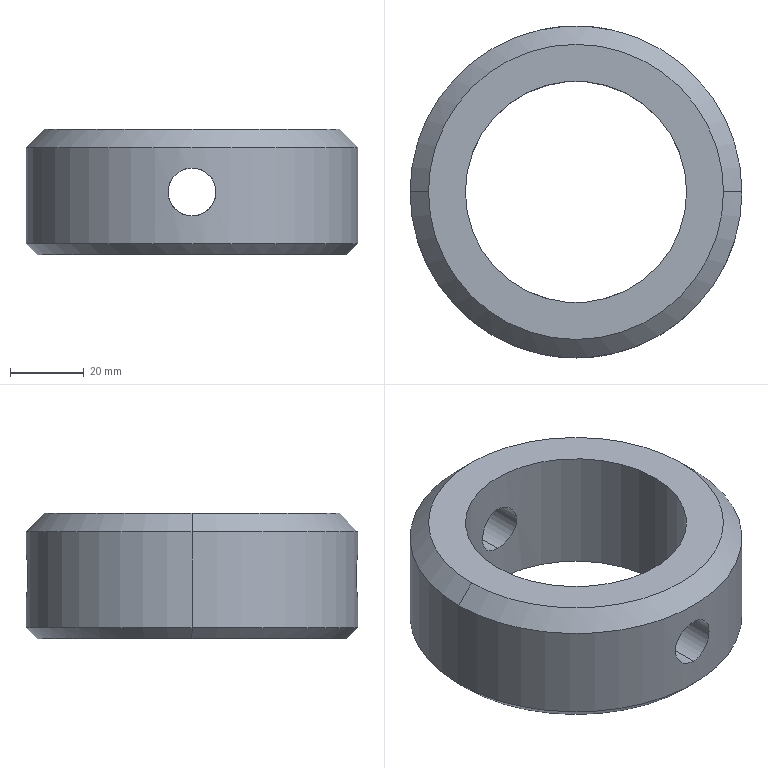Part | SolidWorks | features Chamfer 2, Extrusion 1, ICE 1 | 1 solid | 14 faces | box 90 x 90 x 34 mm | volume 111520 mm3 | cylinder 8 | cone 4 | plane 2 | commonest cylinder face diameters 13 x4 60 x2 90 x2
STEP:
#1=CARTESIAN_POINT('',(-42.,0.,0.));
#2=VERTEX_POINT('',#1);
#3=CARTESIAN_POINT('',(42.,0.,0.));
#4=VERTEX_POINT('',#3);
#5=CARTESIAN_POINT('',(0.,0.,0.));
#6=DIRECTION('',(0.,0.,-1.));
#7=DIRECTION('',(1.,0.,0.));
#8=AXIS2_PLACEMENT_3D('',#5,#6,#7);
#9=CIRCLE('',#8,42.);
#10=EDGE_CURVE('',#2,#4,#9,.T.);
#11=ORIENTED_EDGE('',*,*,#10,.F.);
#12=CARTESIAN_POINT('',(-45.,0.,3.));
#13=VERTEX_POINT('',#12);
#14=CARTESIAN_POINT('',(-45.,0.,3.));
#15=DIRECTION('',(-0.7071,0.,0.7071));
#16=VECTOR('',#15,1000.);
#17=LINE('',#14,#16);
#18=EDGE_CURVE('',#2,#13,#17,.T.);
#19=ORIENTED_EDGE('',*,*,#18,.T.);
#20=CARTESIAN_POINT('',(45.,0.,3.));
#21=VERTEX_POINT('',#20);
#22=CARTESIAN_POINT('',(0.,0.,3.));
#23=DIRECTION('',(0.,0.,1.));
#24=DIRECTION('',(1.,0.,0.));
#25=AXIS2_PLACEMENT_3D('',#22,#23,#24);
#26=CIRCLE('',#25,45.);
#27=EDGE_CURVE('',#21,#13,#26,.T.);
#28=ORIENTED_EDGE('',*,*,#27,.F.);
#29=CARTESIAN_POINT('',(45.,0.,3.));
#30=DIRECTION('',(0.7071,0.,0.7071));
#31=VECTOR('',#30,1000.);
#32=LINE('',#29,#31);
#33=EDGE_CURVE('',#4,#21,#32,.T.);
#34=ORIENTED_EDGE('',*,*,#33,.F.);
#35=EDGE_LOOP('',(#11,#19,#28,#34));
#36=FACE_OUTER_BOUND('',#35,.T.);
#37=CARTESIAN_POINT('',(0.,0.,3.));
#38=DIRECTION('',(0.,0.,1.));
#39=DIRECTION('',(1.,0.,0.));
#40=AXIS2_PLACEMENT_3D('',#37,#38,#39);
#41=CONICAL_SURFACE('',#40,45.,0.7854);
#42=ADVANCED_FACE('',(#36),#41,.T.);
#43=CARTESIAN_POINT('',(40.,0.,34.));
#44=VERTEX_POINT('',#43);
#45=CARTESIAN_POINT('',(-40.,0.,34.));
#46=VERTEX_POINT('',#45);
#47=CARTESIAN_POINT('',(0.,0.,34.));
#48=DIRECTION('',(0.,0.,1.));
#49=DIRECTION('',(1.,0.,0.));
#50=AXIS2_PLACEMENT_3D('',#47,#48,#49);
#51=CIRCLE('',#50,40.);
#52=EDGE_CURVE('',#44,#46,#51,.T.);
#53=ORIENTED_EDGE('',*,*,#52,.F.);
#54=CARTESIAN_POINT('',(45.,0.,29.));
#55=VERTEX_POINT('',#54);
#56=CARTESIAN_POINT('',(40.,0.,34.));
#57=DIRECTION('',(0.7071,0.,-0.7071));
#58=VECTOR('',#57,1000.);
#59=LINE('',#56,#58);
#60=EDGE_CURVE('',#44,#55,#59,.T.);
#61=ORIENTED_EDGE('',*,*,#60,.T.);
#62=CARTESIAN_POINT('',(-45.,0.,29.));
#63=VERTEX_POINT('',#62);
#64=CARTESIAN_POINT('',(0.,0.,29.));
#65=DIRECTION('',(0.,0.,-1.));
#66=DIRECTION('',(1.,0.,0.));
#67=AXIS2_PLACEMENT_3D('',#64,#65,#66);
#68=CIRCLE('',#67,45.);
#69=EDGE_CURVE('',#63,#55,#68,.T.);
#70=ORIENTED_EDGE('',*,*,#69,.F.);
#71=CARTESIAN_POINT('',(-40.,0.,34.));
#72=DIRECTION('',(-0.7071,0.,-0.7071));
#73=VECTOR('',#72,1000.);
#74=LINE('',#71,#73);
#75=EDGE_CURVE('',#46,#63,#74,.T.);
#76=ORIENTED_EDGE('',*,*,#75,.F.);
#77=EDGE_LOOP('',(#53,#61,#70,#76));
#78=FACE_OUTER_BOUND('',#77,.T.);
#79=CARTESIAN_POINT('',(0.,0.,34.));
#80=DIRECTION('',(0.,0.,-1.));
#81=DIRECTION('',(-1.,0.,0.));
#82=AXIS2_PLACEMENT_3D('',#79,#80,#81);
#83=CONICAL_SURFACE('',#82,40.,0.7854);
#84=ADVANCED_FACE('',(#78),#83,.T.);
#85=CARTESIAN_POINT('',(0.,-45.,10.5));
#86=VERTEX_POINT('',#85);
#87=CARTESIAN_POINT('',(0.,-45.,23.5));
#88=VERTEX_POINT('',#87);
#89=CARTESIAN_POINT('',(0.,-45.,10.5));
#90=CARTESIAN_POINT('',(-0.4244,-45.,10.5));
#91=CARTESIAN_POINT('',(-0.8466,-44.994,10.541));
#92=CARTESIAN_POINT('',(-1.477,-44.976,10.666));
#93=CARTESIAN_POINT('',(-1.685,-44.969,10.719));
#94=CARTESIAN_POINT('',(-2.092,-44.952,10.842));
#95=CARTESIAN_POINT('',(-2.491,-44.932,10.985));
#96=CARTESIAN_POINT('',(-2.875,-44.908,11.166));
#97=CARTESIAN_POINT('',(-3.25,-44.883,11.367));
#98=CARTESIAN_POINT('',(-3.434,-44.869,11.477));
#99=CARTESIAN_POINT('',(-3.967,-44.826,11.833));
#100=CARTESIAN_POINT('',(-4.293,-44.796,12.101));
#101=CARTESIAN_POINT('',(-4.893,-44.734,12.7));
#102=CARTESIAN_POINT('',(-5.167,-44.703,13.034));
#103=CARTESIAN_POINT('',(-5.639,-44.646,13.739));
#104=CARTESIAN_POINT('',(-5.839,-44.62,14.112));
#105=CARTESIAN_POINT('',(-6.084,-44.587,14.702));
#106=CARTESIAN_POINT('',(-6.157,-44.577,14.905));
#107=CARTESIAN_POINT('',(-6.281,-44.56,15.313));
#108=CARTESIAN_POINT('',(-6.333,-44.552,15.519));
#109=CARTESIAN_POINT('',(-6.457,-44.534,16.143));
#110=CARTESIAN_POINT('',(-6.5,-44.528,16.566));
#111=CARTESIAN_POINT('',(-6.5,-44.528,17.425));
#112=CARTESIAN_POINT('',(-6.458,-44.534,17.848));
#113=CARTESIAN_POINT('',(-6.335,-44.552,18.472));
#114=CARTESIAN_POINT('',(-6.283,-44.559,18.678));
#115=CARTESIAN_POINT('',(-6.16,-44.576,19.087));
#116=CARTESIAN_POINT('',(-6.087,-44.586,19.29));
#117=CARTESIAN_POINT('',(-5.843,-44.619,19.88));
#118=CARTESIAN_POINT('',(-5.643,-44.645,20.253));
#119=CARTESIAN_POINT('',(-5.172,-44.702,20.96));
#120=CARTESIAN_POINT('',(-4.898,-44.734,21.294));
#121=CARTESIAN_POINT('',(-4.3,-44.795,21.893));
#122=CARTESIAN_POINT('',(-3.974,-44.826,22.162));
#123=CARTESIAN_POINT('',(-3.263,-44.883,22.638));
#124=CARTESIAN_POINT('',(-2.887,-44.909,22.839));
#125=CARTESIAN_POINT('',(-2.3,-44.942,23.083));
#126=CARTESIAN_POINT('',(-2.101,-44.951,23.155));
#127=CARTESIAN_POINT('',(-1.694,-44.969,23.279));
#128=CARTESIAN_POINT('',(-1.485,-44.976,23.332));
#129=CARTESIAN_POINT('',(-0.8549,-44.994,23.458));
#130=CARTESIAN_POINT('',(-0.43,-45.,23.5));
#131=CARTESIAN_POINT('',(0.,-45.,23.5));
#132=B_SPLINE_CURVE_WITH_KNOTS('',3,(#89,#90,#91,#92,#93,#94,#95,#96,#97,#98,#99,#100,#101,#102,#103,#104,#105,#106,#107,#108,#109,#110,#111,#112,#113,#114,#115,#116,#117,#118,#119,#120,#121,#122,#123,#124,#125,#126,#127,#128,#129,#130,#131),.UNSPECIFIED.,.F.,.F.,(4,2,2,1,2,2,2,2,2,2,2,2,2,2,2,2,2,2,2,2,2,4),(0.02035,0.02162,0.02226,0.02289,0.02353,0.02416,0.02543,0.02671,0.02798,0.02861,0.02925,0.03052,0.03179,0.03243,0.03306,0.03433,0.03561,0.03688,0.03815,0.03878,0.03942,0.04069),.UNSPECIFIED.);
#133=EDGE_CURVE('',#86,#88,#132,.T.);
#134=ORIENTED_EDGE('',*,*,#133,.F.);
#135=CARTESIAN_POINT('',(0.,-30.,10.5));
#136=VERTEX_POINT('',#135);
#137=CARTESIAN_POINT('',(0.,-45.,10.5));
#138=DIRECTION('',(0.,1.,0.));
#139=VECTOR('',#138,1000.);
#140=LINE('',#137,#139);
#141=EDGE_CURVE('',#86,#136,#140,.T.);
#142=ORIENTED_EDGE('',*,*,#141,.T.);
#143=CARTESIAN_POINT('',(0.,-30.,23.5));
#144=VERTEX_POINT('',#143);
#145=CARTESIAN_POINT('',(0.,-30.,10.5));
#146=CARTESIAN_POINT('',(-0.4248,-30.,10.5));
#147=CARTESIAN_POINT('',(-0.848,-29.991,10.541));
#148=CARTESIAN_POINT('',(-1.691,-29.955,10.709));
#149=CARTESIAN_POINT('',(-2.099,-29.929,10.834));
#150=CARTESIAN_POINT('',(-2.686,-29.88,11.077));
#151=CARTESIAN_POINT('',(-2.877,-29.862,11.168));
#152=CARTESIAN_POINT('',(-3.253,-29.824,11.369));
#153=CARTESIAN_POINT('',(-3.438,-29.803,11.479));
#154=CARTESIAN_POINT('',(-3.968,-29.739,11.834));
#155=CARTESIAN_POINT('',(-4.294,-29.693,12.102));
#156=CARTESIAN_POINT('',(-4.894,-29.6,12.701));
#157=CARTESIAN_POINT('',(-5.167,-29.553,13.034));
#158=CARTESIAN_POINT('',(-5.638,-29.466,13.737));
#159=CARTESIAN_POINT('',(-5.838,-29.427,14.11));
#160=CARTESIAN_POINT('',(-6.084,-29.377,14.702));
#161=CARTESIAN_POINT('',(-6.157,-29.362,14.904));
#162=CARTESIAN_POINT('',(-6.281,-29.335,15.312));
#163=CARTESIAN_POINT('',(-6.384,-29.313,15.723));
#164=CARTESIAN_POINT('',(-6.447,-29.299,16.143));
#165=CARTESIAN_POINT('',(-6.489,-29.29,16.567));
#166=CARTESIAN_POINT('',(-6.5,-29.287,16.783));
#167=CARTESIAN_POINT('',(-6.5,-29.287,17.426));
#168=CARTESIAN_POINT('',(-6.458,-29.297,17.849));
#169=CARTESIAN_POINT('',(-6.293,-29.333,18.682));
#170=CARTESIAN_POINT('',(-6.167,-29.36,19.097));
#171=CARTESIAN_POINT('',(-5.842,-29.426,19.882));
#172=CARTESIAN_POINT('',(-5.642,-29.466,20.255));
#173=CARTESIAN_POINT('',(-5.288,-29.531,20.786));
#174=CARTESIAN_POINT('',(-5.16,-29.553,20.959));
#175=CARTESIAN_POINT('',(-4.89,-29.599,21.287));
#176=CARTESIAN_POINT('',(-4.748,-29.622,21.444));
#177=CARTESIAN_POINT('',(-4.301,-29.692,21.892));
#178=CARTESIAN_POINT('',(-3.973,-29.738,22.162));
#179=CARTESIAN_POINT('',(-3.262,-29.824,22.638));
#180=CARTESIAN_POINT('',(-2.889,-29.863,22.838));
#181=CARTESIAN_POINT('',(-2.303,-29.912,23.082));
#182=CARTESIAN_POINT('',(-2.103,-29.927,23.154));
#183=CARTESIAN_POINT('',(-1.694,-29.953,23.279));
#184=CARTESIAN_POINT('',(-1.485,-29.964,23.332));
#185=CARTESIAN_POINT('',(-0.8557,-29.991,23.458));
#186=CARTESIAN_POINT('',(-0.4307,-30.,23.5));
#187=CARTESIAN_POINT('',(0.,-30.,23.5));
#188=B_SPLINE_CURVE_WITH_KNOTS('',3,(#145,#146,#147,#148,#149,#150,#151,#152,#153,#154,#155,#156,#157,#158,#159,#160,#161,#162,#163,#164,#165,#166,#167,#168,#169,#170,#171,#172,#173,#174,#175,#176,#177,#178,#179,#180,#181,#182,#183,#184,#185,#186,#187),.UNSPECIFIED.,.F.,.F.,(4,2,2,2,2,2,2,2,2,1,2,2,2,2,2,2,2,2,2,2,2,4),(0.02038,0.02166,0.02293,0.02357,0.0242,0.02548,0.02675,0.02802,0.02866,0.0293,0.02993,0.03057,0.03184,0.03312,0.03439,0.03503,0.03567,0.03694,0.03821,0.03885,0.03949,0.04076),.UNSPECIFIED.);
#189=EDGE_CURVE('',#136,#144,#188,.T.);
#190=ORIENTED_EDGE('',*,*,#189,.T.);
#191=CARTESIAN_POINT('',(0.,-45.,23.5));
#192=DIRECTION('',(0.,1.,0.));
#193=VECTOR('',#192,1000.);
#194=LINE('',#191,#193);
#195=EDGE_CURVE('',#88,#144,#194,.T.);
#196=ORIENTED_EDGE('',*,*,#195,.F.);
#197=EDGE_LOOP('',(#134,#142,#190,#196));
#198=FACE_OUTER_BOUND('',#197,.T.);
#199=CARTESIAN_POINT('',(0.,-45.,17.));
#200=DIRECTION('',(0.,1.,0.));
#201=DIRECTION('',(0.,0.,1.));
#202=AXIS2_PLACEMENT_3D('',#199,#200,#201);
#203=CYLINDRICAL_SURFACE('',#202,6.5);
#204=ADVANCED_FACE('',(#198),#203,.F.);
#205=CARTESIAN_POINT('',(0.,30.,23.5));
#206=VERTEX_POINT('',#205);
#207=CARTESIAN_POINT('',(0.,30.,10.5));
#208=VERTEX_POINT('',#207);
#209=CARTESIAN_POINT('',(0.,30.,23.5));
#210=CARTESIAN_POINT('',(-0.4308,30.,23.5));
#211=CARTESIAN_POINT('',(-0.8542,29.991,23.458));
#212=CARTESIAN_POINT('',(-1.479,29.964,23.333));
#213=CARTESIAN_POINT('',(-1.685,29.953,23.281));
#214=CARTESIAN_POINT('',(-2.094,29.928,23.157));
#215=CARTESIAN_POINT('',(-2.297,29.913,23.084));
#216=CARTESIAN_POINT('',(-2.887,29.863,22.839));
#217=CARTESIAN_POINT('',(-3.26,29.824,22.639));
#218=CARTESIAN_POINT('',(-3.966,29.739,22.168));
#219=CARTESIAN_POINT('',(-4.299,29.692,21.894));
#220=CARTESIAN_POINT('',(-4.896,29.599,21.296));
#221=CARTESIAN_POINT('',(-5.165,29.553,20.97));
#222=CARTESIAN_POINT('',(-5.64,29.466,20.259));
#223=CARTESIAN_POINT('',(-5.841,29.426,19.883));
#224=CARTESIAN_POINT('',(-6.084,29.377,19.297));
#225=CARTESIAN_POINT('',(-6.156,29.362,19.097));
#226=CARTESIAN_POINT('',(-6.28,29.335,18.69));
#227=CARTESIAN_POINT('',(-6.333,29.324,18.48));
#228=CARTESIAN_POINT('',(-6.458,29.297,17.851));
#229=CARTESIAN_POINT('',(-6.5,29.287,17.428));
#230=CARTESIAN_POINT('',(-6.5,29.287,16.577));
#231=CARTESIAN_POINT('',(-6.458,29.297,16.145));
#232=CARTESIAN_POINT('',(-6.291,29.333,15.31));
#233=CARTESIAN_POINT('',(-6.168,29.36,14.905));
#234=CARTESIAN_POINT('',(-5.923,29.41,14.313));
#235=CARTESIAN_POINT('',(-5.83,29.428,14.118));
#236=CARTESIAN_POINT('',(-5.629,29.467,13.743));
#237=CARTESIAN_POINT('',(-5.52,29.488,13.562));
#238=CARTESIAN_POINT('',(-5.168,29.553,13.035));
#239=CARTESIAN_POINT('',(-4.897,29.599,12.705));
#240=CARTESIAN_POINT('',(-4.294,29.693,12.101));
#241=CARTESIAN_POINT('',(-3.967,29.739,11.834));
#242=CARTESIAN_POINT('',(-3.44,29.803,11.481));
#243=CARTESIAN_POINT('',(-3.258,29.823,11.371));
#244=CARTESIAN_POINT('',(-2.881,29.862,11.169));
#245=CARTESIAN_POINT('',(-2.687,29.88,11.077));
#246=CARTESIAN_POINT('',(-2.098,29.929,10.833));
#247=CARTESIAN_POINT('',(-1.692,29.955,10.71));
#248=CARTESIAN_POINT('',(-1.065,29.982,10.584));
#249=CARTESIAN_POINT('',(-0.852,29.989,10.553));
#250=CARTESIAN_POINT('',(-0.4254,29.998,10.51));
#251=CARTESIAN_POINT('',(-0.2125,30.,10.5));
#252=CARTESIAN_POINT('',(0.,30.,10.5));
#253=B_SPLINE_CURVE_WITH_KNOTS('',3,(#209,#210,#211,#212,#213,#214,#215,#216,#217,#218,#219,#220,#221,#222,#223,#224,#225,#226,#227,#228,#229,#230,#231,#232,#233,#234,#235,#236,#237,#238,#239,#240,#241,#242,#243,#244,#245,#246,#247,#248,#249,#250,#251,#252),.UNSPECIFIED.,.F.,.F.,(4,2,2,2,2,2,2,2,2,2,2,2,2,2,2,2,2,2,2,2,2,4),(0.,0.001274,0.001911,0.002548,0.003822,0.005096,0.00637,0.007643,0.00828,0.008917,0.01019,0.01147,0.01274,0.01338,0.01401,0.01529,0.01656,0.0172,0.01783,0.01911,0.01975,0.02038),.UNSPECIFIED.);
#254=EDGE_CURVE('',#206,#208,#253,.T.);
#255=ORIENTED_EDGE('',*,*,#254,.T.);
#256=CARTESIAN_POINT('',(0.,45.,10.5));
#257=VERTEX_POINT('',#256);
#258=CARTESIAN_POINT('',(0.,-45.,10.5));
#259=DIRECTION('',(0.,1.,0.));
#260=VECTOR('',#259,1000.);
#261=LINE('',#258,#260);
#262=EDGE_CURVE('',#208,#257,#261,.T.);
#263=ORIENTED_EDGE('',*,*,#262,.T.);
#264=CARTESIAN_POINT('',(0.,45.,23.5));
#265=VERTEX_POINT('',#264);
#266=CARTESIAN_POINT('',(0.,45.,23.5));
#267=CARTESIAN_POINT('',(-0.4301,45.,23.5));
#268=CARTESIAN_POINT('',(-0.8529,44.994,23.458));
#269=CARTESIAN_POINT('',(-1.477,44.976,23.334));
#270=CARTESIAN_POINT('',(-1.683,44.969,23.282));
#271=CARTESIAN_POINT('',(-2.091,44.952,23.158));
#272=CARTESIAN_POINT('',(-2.294,44.942,23.085));
#273=CARTESIAN_POINT('',(-2.885,44.909,22.84));
#274=CARTESIAN_POINT('',(-3.258,44.883,22.641));
#275=CARTESIAN_POINT('',(-3.964,44.826,22.169));
#276=CARTESIAN_POINT('',(-4.298,44.795,21.895));
#277=CARTESIAN_POINT('',(-4.897,44.734,21.296));
#278=CARTESIAN_POINT('',(-5.165,44.703,20.969));
#279=CARTESIAN_POINT('',(-5.522,44.66,20.436));
#280=CARTESIAN_POINT('',(-5.632,44.646,20.252));
#281=CARTESIAN_POINT('',(-5.833,44.621,19.877));
#282=CARTESIAN_POINT('',(-6.014,44.597,19.494));
#283=CARTESIAN_POINT('',(-6.157,44.577,19.095));
#284=CARTESIAN_POINT('',(-6.281,44.56,18.688));
#285=CARTESIAN_POINT('',(-6.333,44.552,18.479));
#286=CARTESIAN_POINT('',(-6.458,44.534,17.849));
#287=CARTESIAN_POINT('',(-6.5,44.528,17.427));
#288=CARTESIAN_POINT('',(-6.5,44.528,16.578));
#289=CARTESIAN_POINT('',(-6.458,44.534,16.147));
#290=CARTESIAN_POINT('',(-6.291,44.558,15.312));
#291=CARTESIAN_POINT('',(-6.169,44.576,14.907));
#292=CARTESIAN_POINT('',(-5.924,44.608,14.316));
#293=CARTESIAN_POINT('',(-5.832,44.621,14.121));
#294=CARTESIAN_POINT('',(-5.631,44.646,13.745));
#295=CARTESIAN_POINT('',(-5.521,44.66,13.564));
#296=CARTESIAN_POINT('',(-5.169,44.703,13.036));
#297=CARTESIAN_POINT('',(-4.899,44.734,12.707));
#298=CARTESIAN_POINT('',(-4.294,44.796,12.101));
#299=CARTESIAN_POINT('',(-3.966,44.826,11.833));
#300=CARTESIAN_POINT('',(-3.438,44.869,11.48));
#301=CARTESIAN_POINT('',(-3.256,44.882,11.37));
#302=CARTESIAN_POINT('',(-2.88,44.908,11.169));
#303=CARTESIAN_POINT('',(-2.685,44.92,11.077));
#304=CARTESIAN_POINT('',(-2.095,44.953,10.832));
#305=CARTESIAN_POINT('',(-1.69,44.97,10.709));
#306=CARTESIAN_POINT('',(-0.8557,44.994,10.543));
#307=CARTESIAN_POINT('',(-0.4245,45.,10.5));
#308=CARTESIAN_POINT('',(0.,45.,10.5));
#309=B_SPLINE_CURVE_WITH_KNOTS('',3,(#266,#267,#268,#269,#270,#271,#272,#273,#274,#275,#276,#277,#278,#279,#280,#281,#282,#283,#284,#285,#286,#287,#288,#289,#290,#291,#292,#293,#294,#295,#296,#297,#298,#299,#300,#301,#302,#303,#304,#305,#306,#307,#308),.UNSPECIFIED.,.F.,.F.,(4,2,2,2,2,2,2,2,1,2,2,2,2,2,2,2,2,2,2,2,2,4),(0.,0.001272,0.001908,0.002544,0.003815,0.005087,0.006359,0.006995,0.007631,0.008267,0.008903,0.01017,0.01145,0.01272,0.01335,0.01399,0.01526,0.01653,0.01717,0.01781,0.01908,0.02035),.UNSPECIFIED.);
#310=EDGE_CURVE('',#265,#257,#309,.T.);
#311=ORIENTED_EDGE('',*,*,#310,.F.);
#312=CARTESIAN_POINT('',(0.,-45.,23.5));
#313=DIRECTION('',(0.,1.,0.));
#314=VECTOR('',#313,1000.);
#315=LINE('',#312,#314);
#316=EDGE_CURVE('',#206,#265,#315,.T.);
#317=ORIENTED_EDGE('',*,*,#316,.F.);
#318=EDGE_LOOP('',(#255,#263,#311,#317));
#319=FACE_OUTER_BOUND('',#318,.T.);
#320=CARTESIAN_POINT('',(0.,-45.,17.));
#321=DIRECTION('',(0.,1.,0.));
#322=DIRECTION('',(0.,0.,1.));
#323=AXIS2_PLACEMENT_3D('',#320,#321,#322);
#324=CYLINDRICAL_SURFACE('',#323,6.5);
#325=ADVANCED_FACE('',(#319),#324,.F.);
#326=CARTESIAN_POINT('',(0.,-30.,23.5));
#327=CARTESIAN_POINT('',(0.4308,-30.,23.5));
#328=CARTESIAN_POINT('',(0.8542,-29.991,23.458));
#329=CARTESIAN_POINT('',(1.479,-29.964,23.333));
#330=CARTESIAN_POINT('',(1.685,-29.953,23.281));
#331=CARTESIAN_POINT('',(2.094,-29.928,23.157));
#332=CARTESIAN_POINT('',(2.297,-29.913,23.084));
#333=CARTESIAN_POINT('',(2.887,-29.863,22.839));
#334=CARTESIAN_POINT('',(3.26,-29.824,22.639));
#335=CARTESIAN_POINT('',(3.966,-29.739,22.168));
#336=CARTESIAN_POINT('',(4.299,-29.692,21.894));
#337=CARTESIAN_POINT('',(4.896,-29.599,21.296));
#338=CARTESIAN_POINT('',(5.165,-29.553,20.97));
#339=CARTESIAN_POINT('',(5.64,-29.466,20.259));
#340=CARTESIAN_POINT('',(5.841,-29.426,19.883));
#341=CARTESIAN_POINT('',(6.084,-29.377,19.297));
#342=CARTESIAN_POINT('',(6.156,-29.362,19.097));
#343=CARTESIAN_POINT('',(6.28,-29.335,18.69));
#344=CARTESIAN_POINT('',(6.333,-29.324,18.48));
#345=CARTESIAN_POINT('',(6.458,-29.297,17.851));
#346=CARTESIAN_POINT('',(6.5,-29.287,17.428));
#347=CARTESIAN_POINT('',(6.5,-29.287,16.577));
#348=CARTESIAN_POINT('',(6.458,-29.297,16.145));
#349=CARTESIAN_POINT('',(6.291,-29.333,15.31));
#350=CARTESIAN_POINT('',(6.168,-29.36,14.905));
#351=CARTESIAN_POINT('',(5.923,-29.41,14.313));
#352=CARTESIAN_POINT('',(5.83,-29.428,14.118));
#353=CARTESIAN_POINT('',(5.629,-29.467,13.743));
#354=CARTESIAN_POINT('',(5.52,-29.488,13.562));
#355=CARTESIAN_POINT('',(5.168,-29.553,13.035));
#356=CARTESIAN_POINT('',(4.897,-29.599,12.705));
#357=CARTESIAN_POINT('',(4.294,-29.693,12.101));
#358=CARTESIAN_POINT('',(3.967,-29.739,11.834));
#359=CARTESIAN_POINT('',(3.44,-29.803,11.481));
#360=CARTESIAN_POINT('',(3.258,-29.823,11.371));
#361=CARTESIAN_POINT('',(2.881,-29.862,11.169));
#362=CARTESIAN_POINT('',(2.687,-29.88,11.077));
#363=CARTESIAN_POINT('',(2.098,-29.929,10.833));
#364=CARTESIAN_POINT('',(1.692,-29.955,10.71));
#365=CARTESIAN_POINT('',(1.065,-29.982,10.584));
#366=CARTESIAN_POINT('',(0.852,-29.989,10.553));
#367=CARTESIAN_POINT('',(0.4254,-29.998,10.51));
#368=CARTESIAN_POINT('',(0.2125,-30.,10.5));
#369=CARTESIAN_POINT('',(0.,-30.,10.5));
#370=B_SPLINE_CURVE_WITH_KNOTS('',3,(#326,#327,#328,#329,#330,#331,#332,#333,#334,#335,#336,#337,#338,#339,#340,#341,#342,#343,#344,#345,#346,#347,#348,#349,#350,#351,#352,#353,#354,#355,#356,#357,#358,#359,#360,#361,#362,#363,#364,#365,#366,#367,#368,#369),.UNSPECIFIED.,.F.,.F.,(4,2,2,2,2,2,2,2,2,2,2,2,2,2,2,2,2,2,2,2,2,4),(0.,0.001274,0.001911,0.002548,0.003822,0.005096,0.00637,0.007643,0.00828,0.008917,0.01019,0.01147,0.01274,0.01338,0.01401,0.01529,0.01656,0.0172,0.01783,0.01911,0.01975,0.02038),.UNSPECIFIED.);
#371=EDGE_CURVE('',#144,#136,#370,.T.);
#372=ORIENTED_EDGE('',*,*,#371,.F.);
#373=ORIENTED_EDGE('',*,*,#189,.F.);
#374=EDGE_LOOP('',(#372,#373));
#375=FACE_BOUND('',#374,.T.);
#376=CARTESIAN_POINT('',(-30.,0.,34.));
#377=VERTEX_POINT('',#376);
#378=CARTESIAN_POINT('',(30.,0.,34.));
#379=VERTEX_POINT('',#378);
#380=CARTESIAN_POINT('',(0.,0.,34.));
#381=DIRECTION('',(0.,0.,1.));
#382=DIRECTION('',(1.,0.,0.));
#383=AXIS2_PLACEMENT_3D('',#380,#381,#382);
#384=CIRCLE('',#383,30.);
#385=EDGE_CURVE('',#377,#379,#384,.T.);
#386=ORIENTED_EDGE('',*,*,#385,.T.);
#387=CARTESIAN_POINT('',(30.,0.,0.));
#388=VERTEX_POINT('',#387);
#389=CARTESIAN_POINT('',(30.,0.,34.));
#390=DIRECTION('',(0.,0.,-1.));
#391=VECTOR('',#390,1000.);
#392=LINE('',#389,#391);
#393=EDGE_CURVE('',#379,#388,#392,.T.);
#394=ORIENTED_EDGE('',*,*,#393,.T.);
#395=CARTESIAN_POINT('',(-30.,0.,0.));
#396=VERTEX_POINT('',#395);
#397=CARTESIAN_POINT('',(0.,0.,0.));
#398=DIRECTION('',(0.,0.,1.));
#399=DIRECTION('',(1.,0.,0.));
#400=AXIS2_PLACEMENT_3D('',#397,#398,#399);
#401=CIRCLE('',#400,30.);
#402=EDGE_CURVE('',#396,#388,#401,.T.);
#403=ORIENTED_EDGE('',*,*,#402,.F.);
#404=CARTESIAN_POINT('',(-30.,0.,34.));
#405=DIRECTION('',(0.,0.,-1.));
#406=VECTOR('',#405,1000.);
#407=LINE('',#404,#406);
#408=EDGE_CURVE('',#377,#396,#407,.T.);
#409=ORIENTED_EDGE('',*,*,#408,.F.);
#410=EDGE_LOOP('',(#386,#394,#403,#409));
#411=FACE_OUTER_BOUND('',#410,.T.);
#412=CARTESIAN_POINT('',(0.,0.,34.));
#413=DIRECTION('',(0.,0.,-1.));
#414=DIRECTION('',(-1.,0.,0.));
#415=AXIS2_PLACEMENT_3D('',#412,#413,#414);
#416=CYLINDRICAL_SURFACE('',#415,30.);
#417=ADVANCED_FACE('',(#375,#411),#416,.F.);
#418=ORIENTED_EDGE('',*,*,#310,.T.);
#419=CARTESIAN_POINT('',(0.,45.,10.5));
#420=CARTESIAN_POINT('',(0.4244,45.,10.5));
#421=CARTESIAN_POINT('',(0.8466,44.994,10.541));
#422=CARTESIAN_POINT('',(1.477,44.976,10.666));
#423=CARTESIAN_POINT('',(1.685,44.969,10.719));
#424=CARTESIAN_POINT('',(2.092,44.952,10.842));
#425=CARTESIAN_POINT('',(2.491,44.932,10.985));
#426=CARTESIAN_POINT('',(2.875,44.908,11.166));
#427=CARTESIAN_POINT('',(3.25,44.883,11.367));
#428=CARTESIAN_POINT('',(3.434,44.869,11.477));
#429=CARTESIAN_POINT('',(3.967,44.826,11.833));
#430=CARTESIAN_POINT('',(4.293,44.796,12.101));
#431=CARTESIAN_POINT('',(4.893,44.734,12.7));
#432=CARTESIAN_POINT('',(5.167,44.703,13.034));
#433=CARTESIAN_POINT('',(5.639,44.646,13.739));
#434=CARTESIAN_POINT('',(5.839,44.62,14.112));
#435=CARTESIAN_POINT('',(6.084,44.587,14.702));
#436=CARTESIAN_POINT('',(6.157,44.577,14.905));
#437=CARTESIAN_POINT('',(6.281,44.56,15.313));
#438=CARTESIAN_POINT('',(6.333,44.552,15.519));
#439=CARTESIAN_POINT('',(6.457,44.534,16.143));
#440=CARTESIAN_POINT('',(6.5,44.528,16.566));
#441=CARTESIAN_POINT('',(6.5,44.528,17.425));
#442=CARTESIAN_POINT('',(6.458,44.534,17.848));
#443=CARTESIAN_POINT('',(6.335,44.552,18.472));
#444=CARTESIAN_POINT('',(6.283,44.559,18.678));
#445=CARTESIAN_POINT('',(6.16,44.576,19.087));
#446=CARTESIAN_POINT('',(6.087,44.586,19.29));
#447=CARTESIAN_POINT('',(5.843,44.619,19.88));
#448=CARTESIAN_POINT('',(5.643,44.645,20.253));
#449=CARTESIAN_POINT('',(5.172,44.702,20.96));
#450=CARTESIAN_POINT('',(4.898,44.734,21.294));
#451=CARTESIAN_POINT('',(4.3,44.795,21.893));
#452=CARTESIAN_POINT('',(3.974,44.826,22.162));
#453=CARTESIAN_POINT('',(3.263,44.883,22.638));
#454=CARTESIAN_POINT('',(2.887,44.909,22.839));
#455=CARTESIAN_POINT('',(2.3,44.942,23.083));
#456=CARTESIAN_POINT('',(2.101,44.951,23.155));
#457=CARTESIAN_POINT('',(1.694,44.969,23.279));
#458=CARTESIAN_POINT('',(1.485,44.976,23.332));
#459=CARTESIAN_POINT('',(0.8549,44.994,23.458));
#460=CARTESIAN_POINT('',(0.43,45.,23.5));
#461=CARTESIAN_POINT('',(0.,45.,23.5));
#462=B_SPLINE_CURVE_WITH_KNOTS('',3,(#419,#420,#421,#422,#423,#424,#425,#426,#427,#428,#429,#430,#431,#432,#433,#434,#435,#436,#437,#438,#439,#440,#441,#442,#443,#444,#445,#446,#447,#448,#449,#450,#451,#452,#453,#454,#455,#456,#457,#458,#459,#460,#461),.UNSPECIFIED.,.F.,.F.,(4,2,2,1,2,2,2,2,2,2,2,2,2,2,2,2,2,2,2,2,2,4),(0.02035,0.02162,0.02226,0.02289,0.02353,0.02416,0.02543,0.02671,0.02798,0.02861,0.02925,0.03052,0.03179,0.03243,0.03306,0.03433,0.03561,0.03688,0.03815,0.03878,0.03942,0.04069),.UNSPECIFIED.);
#463=EDGE_CURVE('',#257,#265,#462,.T.);
#464=ORIENTED_EDGE('',*,*,#463,.T.);
#465=EDGE_LOOP('',(#418,#464));
#466=FACE_BOUND('',#465,.T.);
#467=ORIENTED_EDGE('',*,*,#69,.T.);
#468=CARTESIAN_POINT('',(45.,0.,34.));
#469=DIRECTION('',(0.,0.,-1.));
#470=VECTOR('',#469,1000.);
#471=LINE('',#468,#470);
#472=EDGE_CURVE('',#55,#21,#471,.T.);
#473=ORIENTED_EDGE('',*,*,#472,.T.);
#474=ORIENTED_EDGE('',*,*,#27,.T.);
#475=CARTESIAN_POINT('',(-45.,0.,34.));
#476=DIRECTION('',(0.,0.,-1.));
#477=VECTOR('',#476,1000.);
#478=LINE('',#475,#477);
#479=EDGE_CURVE('',#63,#13,#478,.T.);
#480=ORIENTED_EDGE('',*,*,#479,.F.);
#481=EDGE_LOOP('',(#467,#473,#474,#480));
#482=FACE_OUTER_BOUND('',#481,.T.);
#483=CARTESIAN_POINT('',(0.,0.,34.));
#484=DIRECTION('',(0.,0.,-1.));
#485=DIRECTION('',(-1.,0.,0.));
#486=AXIS2_PLACEMENT_3D('',#483,#484,#485);
#487=CYLINDRICAL_SURFACE('',#486,45.);
#488=ADVANCED_FACE('',(#466,#482),#487,.T.);
#489=CARTESIAN_POINT('',(0.,0.,34.));
#490=DIRECTION('',(0.,0.,1.));
#491=DIRECTION('',(1.,0.,0.));
#492=AXIS2_PLACEMENT_3D('',#489,#490,#491);
#493=CIRCLE('',#492,40.);
#494=EDGE_CURVE('',#46,#44,#493,.T.);
#495=ORIENTED_EDGE('',*,*,#494,.T.);
#496=ORIENTED_EDGE('',*,*,#52,.T.);
#497=EDGE_LOOP('',(#495,#496));
#498=FACE_OUTER_BOUND('',#497,.T.);
#499=ORIENTED_EDGE('',*,*,#385,.F.);
#500=CARTESIAN_POINT('',(0.,0.,34.));
#501=DIRECTION('',(0.,0.,1.));
#502=DIRECTION('',(1.,0.,0.));
#503=AXIS2_PLACEMENT_3D('',#500,#501,#502);
#504=CIRCLE('',#503,30.);
#505=EDGE_CURVE('',#379,#377,#504,.T.);
#506=ORIENTED_EDGE('',*,*,#505,.F.);
#507=EDGE_LOOP('',(#499,#506));
#508=FACE_BOUND('',#507,.T.);
#509=CARTESIAN_POINT('',(0.,0.,34.));
#510=DIRECTION('',(0.,0.,1.));
#511=DIRECTION('',(1.,0.,0.));
#512=AXIS2_PLACEMENT_3D('',#509,#510,#511);
#513=PLANE('',#512);
#514=ADVANCED_FACE('',(#498,#508),#513,.T.);
#515=CARTESIAN_POINT('',(0.,0.,0.));
#516=DIRECTION('',(0.,0.,-1.));
#517=DIRECTION('',(1.,0.,0.));
#518=AXIS2_PLACEMENT_3D('',#515,#516,#517);
#519=CIRCLE('',#518,42.);
#520=EDGE_CURVE('',#4,#2,#519,.T.);
#521=ORIENTED_EDGE('',*,*,#520,.T.);
#522=ORIENTED_EDGE('',*,*,#10,.T.);
#523=EDGE_LOOP('',(#521,#522));
#524=FACE_OUTER_BOUND('',#523,.T.);
#525=ORIENTED_EDGE('',*,*,#402,.T.);
#526=CARTESIAN_POINT('',(0.,0.,0.));
#527=DIRECTION('',(0.,0.,1.));
#528=DIRECTION('',(1.,0.,0.));
#529=AXIS2_PLACEMENT_3D('',#526,#527,#528);
#530=CIRCLE('',#529,30.);
#531=EDGE_CURVE('',#388,#396,#530,.T.);
#532=ORIENTED_EDGE('',*,*,#531,.T.);
#533=EDGE_LOOP('',(#525,#532));
#534=FACE_BOUND('',#533,.T.);
#535=CARTESIAN_POINT('',(0.,0.,0.));
#536=DIRECTION('',(0.,0.,1.));
#537=DIRECTION('',(1.,0.,0.));
#538=AXIS2_PLACEMENT_3D('',#535,#536,#537);
#539=PLANE('',#538);
#540=ADVANCED_FACE('',(#524,#534),#539,.F.);
#541=ORIENTED_EDGE('',*,*,#472,.F.);
#542=CARTESIAN_POINT('',(0.,0.,29.));
#543=DIRECTION('',(0.,0.,-1.));
#544=DIRECTION('',(1.,0.,0.));
#545=AXIS2_PLACEMENT_3D('',#542,#543,#544);
#546=CIRCLE('',#545,45.);
#547=EDGE_CURVE('',#55,#63,#546,.T.);
#548=ORIENTED_EDGE('',*,*,#547,.T.);
#549=ORIENTED_EDGE('',*,*,#479,.T.);
#550=CARTESIAN_POINT('',(0.,0.,3.));
#551=DIRECTION('',(0.,0.,1.));
#552=DIRECTION('',(1.,0.,0.));
#553=AXIS2_PLACEMENT_3D('',#550,#551,#552);
#554=CIRCLE('',#553,45.);
#555=EDGE_CURVE('',#13,#21,#554,.T.);
#556=ORIENTED_EDGE('',*,*,#555,.T.);
#557=EDGE_LOOP('',(#541,#548,#549,#556));
#558=FACE_OUTER_BOUND('',#557,.T.);
#559=CARTESIAN_POINT('',(0.,-45.,23.5));
#560=CARTESIAN_POINT('',(0.4301,-45.,23.5));
#561=CARTESIAN_POINT('',(0.8529,-44.994,23.458));
#562=CARTESIAN_POINT('',(1.477,-44.976,23.334));
#563=CARTESIAN_POINT('',(1.683,-44.969,23.282));
#564=CARTESIAN_POINT('',(2.091,-44.952,23.158));
#565=CARTESIAN_POINT('',(2.294,-44.942,23.085));
#566=CARTESIAN_POINT('',(2.885,-44.909,22.84));
#567=CARTESIAN_POINT('',(3.258,-44.883,22.641));
#568=CARTESIAN_POINT('',(3.964,-44.826,22.169));
#569=CARTESIAN_POINT('',(4.298,-44.795,21.895));
#570=CARTESIAN_POINT('',(4.897,-44.734,21.296));
#571=CARTESIAN_POINT('',(5.165,-44.703,20.969));
#572=CARTESIAN_POINT('',(5.522,-44.66,20.436));
#573=CARTESIAN_POINT('',(5.632,-44.646,20.252));
#574=CARTESIAN_POINT('',(5.833,-44.621,19.877));
#575=CARTESIAN_POINT('',(6.014,-44.597,19.494));
#576=CARTESIAN_POINT('',(6.157,-44.577,19.095));
#577=CARTESIAN_POINT('',(6.281,-44.56,18.688));
#578=CARTESIAN_POINT('',(6.333,-44.552,18.479));
#579=CARTESIAN_POINT('',(6.458,-44.534,17.849));
#580=CARTESIAN_POINT('',(6.5,-44.528,17.427));
#581=CARTESIAN_POINT('',(6.5,-44.528,16.578));
#582=CARTESIAN_POINT('',(6.458,-44.534,16.147));
#583=CARTESIAN_POINT('',(6.291,-44.558,15.312));
#584=CARTESIAN_POINT('',(6.169,-44.576,14.907));
#585=CARTESIAN_POINT('',(5.924,-44.608,14.316));
#586=CARTESIAN_POINT('',(5.832,-44.621,14.121));
#587=CARTESIAN_POINT('',(5.631,-44.646,13.745));
#588=CARTESIAN_POINT('',(5.521,-44.66,13.564));
#589=CARTESIAN_POINT('',(5.169,-44.703,13.036));
#590=CARTESIAN_POINT('',(4.899,-44.734,12.707));
#591=CARTESIAN_POINT('',(4.294,-44.796,12.101));
#592=CARTESIAN_POINT('',(3.966,-44.826,11.833));
#593=CARTESIAN_POINT('',(3.438,-44.869,11.48));
#594=CARTESIAN_POINT('',(3.256,-44.882,11.37));
#595=CARTESIAN_POINT('',(2.88,-44.908,11.169));
#596=CARTESIAN_POINT('',(2.685,-44.92,11.077));
#597=CARTESIAN_POINT('',(2.095,-44.953,10.832));
#598=CARTESIAN_POINT('',(1.69,-44.97,10.709));
#599=CARTESIAN_POINT('',(0.8557,-44.994,10.543));
#600=CARTESIAN_POINT('',(0.4245,-45.,10.5));
#601=CARTESIAN_POINT('',(0.,-45.,10.5));
#602=B_SPLINE_CURVE_WITH_KNOTS('',3,(#559,#560,#561,#562,#563,#564,#565,#566,#567,#568,#569,#570,#571,#572,#573,#574,#575,#576,#577,#578,#579,#580,#581,#582,#583,#584,#585,#586,#587,#588,#589,#590,#591,#592,#593,#594,#595,#596,#597,#598,#599,#600,#601),.UNSPECIFIED.,.F.,.F.,(4,2,2,2,2,2,2,2,1,2,2,2,2,2,2,2,2,2,2,2,2,4),(0.,0.001272,0.001908,0.002544,0.003815,0.005087,0.006359,0.006995,0.007631,0.008267,0.008903,0.01017,0.01145,0.01272,0.01335,0.01399,0.01526,0.01653,0.01717,0.01781,0.01908,0.02035),.UNSPECIFIED.);
#603=EDGE_CURVE('',#88,#86,#602,.T.);
#604=ORIENTED_EDGE('',*,*,#603,.T.);
#605=ORIENTED_EDGE('',*,*,#133,.T.);
#606=EDGE_LOOP('',(#604,#605));
#607=FACE_BOUND('',#606,.T.);
#608=CARTESIAN_POINT('',(0.,0.,34.));
#609=DIRECTION('',(0.,0.,-1.));
#610=DIRECTION('',(-1.,0.,0.));
#611=AXIS2_PLACEMENT_3D('',#608,#609,#610);
#612=CYLINDRICAL_SURFACE('',#611,45.);
#613=ADVANCED_FACE('',(#558,#607),#612,.T.);
#614=ORIENTED_EDGE('',*,*,#393,.F.);
#615=ORIENTED_EDGE('',*,*,#505,.T.);
#616=ORIENTED_EDGE('',*,*,#408,.T.);
#617=ORIENTED_EDGE('',*,*,#531,.F.);
#618=EDGE_LOOP('',(#614,#615,#616,#617));
#619=FACE_OUTER_BOUND('',#618,.T.);
#620=ORIENTED_EDGE('',*,*,#254,.F.);
#621=CARTESIAN_POINT('',(0.,30.,10.5));
#622=CARTESIAN_POINT('',(0.4248,30.,10.5));
#623=CARTESIAN_POINT('',(0.848,29.991,10.541));
#624=CARTESIAN_POINT('',(1.691,29.955,10.709));
#625=CARTESIAN_POINT('',(2.099,29.929,10.834));
#626=CARTESIAN_POINT('',(2.686,29.88,11.077));
#627=CARTESIAN_POINT('',(2.877,29.862,11.168));
#628=CARTESIAN_POINT('',(3.253,29.824,11.369));
#629=CARTESIAN_POINT('',(3.438,29.803,11.479));
#630=CARTESIAN_POINT('',(3.968,29.739,11.834));
#631=CARTESIAN_POINT('',(4.294,29.693,12.102));
#632=CARTESIAN_POINT('',(4.894,29.6,12.701));
#633=CARTESIAN_POINT('',(5.167,29.553,13.034));
#634=CARTESIAN_POINT('',(5.638,29.466,13.737));
#635=CARTESIAN_POINT('',(5.838,29.427,14.11));
#636=CARTESIAN_POINT('',(6.084,29.377,14.702));
#637=CARTESIAN_POINT('',(6.157,29.362,14.904));
#638=CARTESIAN_POINT('',(6.281,29.335,15.312));
#639=CARTESIAN_POINT('',(6.384,29.313,15.723));
#640=CARTESIAN_POINT('',(6.447,29.299,16.143));
#641=CARTESIAN_POINT('',(6.489,29.29,16.567));
#642=CARTESIAN_POINT('',(6.5,29.287,16.783));
#643=CARTESIAN_POINT('',(6.5,29.287,17.426));
#644=CARTESIAN_POINT('',(6.458,29.297,17.849));
#645=CARTESIAN_POINT('',(6.293,29.333,18.682));
#646=CARTESIAN_POINT('',(6.167,29.36,19.097));
#647=CARTESIAN_POINT('',(5.842,29.426,19.882));
#648=CARTESIAN_POINT('',(5.642,29.466,20.255));
#649=CARTESIAN_POINT('',(5.288,29.531,20.786));
#650=CARTESIAN_POINT('',(5.16,29.553,20.959));
#651=CARTESIAN_POINT('',(4.89,29.599,21.287));
#652=CARTESIAN_POINT('',(4.748,29.622,21.444));
#653=CARTESIAN_POINT('',(4.301,29.692,21.892));
#654=CARTESIAN_POINT('',(3.973,29.738,22.162));
#655=CARTESIAN_POINT('',(3.262,29.824,22.638));
#656=CARTESIAN_POINT('',(2.889,29.863,22.838));
#657=CARTESIAN_POINT('',(2.303,29.912,23.082));
#658=CARTESIAN_POINT('',(2.103,29.927,23.154));
#659=CARTESIAN_POINT('',(1.694,29.953,23.279));
#660=CARTESIAN_POINT('',(1.485,29.964,23.332));
#661=CARTESIAN_POINT('',(0.8557,29.991,23.458));
#662=CARTESIAN_POINT('',(0.4307,30.,23.5));
#663=CARTESIAN_POINT('',(0.,30.,23.5));
#664=B_SPLINE_CURVE_WITH_KNOTS('',3,(#621,#622,#623,#624,#625,#626,#627,#628,#629,#630,#631,#632,#633,#634,#635,#636,#637,#638,#639,#640,#641,#642,#643,#644,#645,#646,#647,#648,#649,#650,#651,#652,#653,#654,#655,#656,#657,#658,#659,#660,#661,#662,#663),.UNSPECIFIED.,.F.,.F.,(4,2,2,2,2,2,2,2,2,1,2,2,2,2,2,2,2,2,2,2,2,4),(0.02038,0.02166,0.02293,0.02357,0.0242,0.02548,0.02675,0.02802,0.02866,0.0293,0.02993,0.03057,0.03184,0.03312,0.03439,0.03503,0.03567,0.03694,0.03821,0.03885,0.03949,0.04076),.UNSPECIFIED.);
#665=EDGE_CURVE('',#208,#206,#664,.T.);
#666=ORIENTED_EDGE('',*,*,#665,.F.);
#667=EDGE_LOOP('',(#620,#666));
#668=FACE_BOUND('',#667,.T.);
#669=CARTESIAN_POINT('',(0.,0.,34.));
#670=DIRECTION('',(0.,0.,-1.));
#671=DIRECTION('',(-1.,0.,0.));
#672=AXIS2_PLACEMENT_3D('',#669,#670,#671);
#673=CYLINDRICAL_SURFACE('',#672,30.);
#674=ADVANCED_FACE('',(#619,#668),#673,.F.);
#675=ORIENTED_EDGE('',*,*,#262,.F.);
#676=ORIENTED_EDGE('',*,*,#665,.T.);
#677=ORIENTED_EDGE('',*,*,#316,.T.);
#678=ORIENTED_EDGE('',*,*,#463,.F.);
#679=EDGE_LOOP('',(#675,#676,#677,#678));
#680=FACE_OUTER_BOUND('',#679,.T.);
#681=CARTESIAN_POINT('',(0.,-45.,17.));
#682=DIRECTION('',(0.,1.,0.));
#683=DIRECTION('',(0.,0.,1.));
#684=AXIS2_PLACEMENT_3D('',#681,#682,#683);
#685=CYLINDRICAL_SURFACE('',#684,6.5);
#686=ADVANCED_FACE('',(#680),#685,.F.);
#687=ORIENTED_EDGE('',*,*,#141,.F.);
#688=ORIENTED_EDGE('',*,*,#603,.F.);
#689=ORIENTED_EDGE('',*,*,#195,.T.);
#690=ORIENTED_EDGE('',*,*,#371,.T.);
#691=EDGE_LOOP('',(#687,#688,#689,#690));
#692=FACE_OUTER_BOUND('',#691,.T.);
#693=CARTESIAN_POINT('',(0.,-45.,17.));
#694=DIRECTION('',(0.,1.,0.));
#695=DIRECTION('',(0.,0.,1.));
#696=AXIS2_PLACEMENT_3D('',#693,#694,#695);
#697=CYLINDRICAL_SURFACE('',#696,6.5);
#698=ADVANCED_FACE('',(#692),#697,.F.);
#699=ORIENTED_EDGE('',*,*,#60,.F.);
#700=ORIENTED_EDGE('',*,*,#494,.F.);
#701=ORIENTED_EDGE('',*,*,#75,.T.);
#702=ORIENTED_EDGE('',*,*,#547,.F.);
#703=EDGE_LOOP('',(#699,#700,#701,#702));
#704=FACE_OUTER_BOUND('',#703,.T.);
#705=CARTESIAN_POINT('',(0.,0.,34.));
#706=DIRECTION('',(0.,0.,-1.));
#707=DIRECTION('',(-1.,0.,0.));
#708=AXIS2_PLACEMENT_3D('',#705,#706,#707);
#709=CONICAL_SURFACE('',#708,40.,0.7854);
#710=ADVANCED_FACE('',(#704),#709,.T.);
#711=ORIENTED_EDGE('',*,*,#18,.F.);
#712=ORIENTED_EDGE('',*,*,#520,.F.);
#713=ORIENTED_EDGE('',*,*,#33,.T.);
#714=ORIENTED_EDGE('',*,*,#555,.F.);
#715=EDGE_LOOP('',(#711,#712,#713,#714));
#716=FACE_OUTER_BOUND('',#715,.T.);
#717=CARTESIAN_POINT('',(0.,0.,3.));
#718=DIRECTION('',(0.,0.,1.));
#719=DIRECTION('',(1.,0.,0.));
#720=AXIS2_PLACEMENT_3D('',#717,#718,#719);
#721=CONICAL_SURFACE('',#720,45.,0.7854);
#722=ADVANCED_FACE('',(#716),#721,.T.);
#723=CLOSED_SHELL('',(#42,#84,#204,#325,#417,#488,#514,#540,#613,#674,#686,#698,#710,#722));
#724=MANIFOLD_SOLID_BREP('',#723);
#725=CARTESIAN_POINT('',(0.,0.,0.));
#726=DIRECTION('',(0.,0.,1.));
#727=DIRECTION('',(1.,0.,0.));
#728=AXIS2_PLACEMENT_3D('',#725,#726,#727);
#729=(LENGTH_UNIT()NAMED_UNIT(*)SI_UNIT(.MILLI.,.METRE.));
#730=UNCERTAINTY_MEASURE_WITH_UNIT(LENGTH_MEASURE(0.00001),#729,'','');
#731=(NAMED_UNIT(*)PLANE_ANGLE_UNIT()SI_UNIT($,.RADIAN.));
#732=(NAMED_UNIT(*)SI_UNIT($,.STERADIAN.)SOLID_ANGLE_UNIT());
#733=(GEOMETRIC_REPRESENTATION_CONTEXT(3)GLOBAL_UNCERTAINTY_ASSIGNED_CONTEXT((#730))GLOBAL_UNIT_ASSIGNED_CONTEXT((#729,#731,#732))REPRESENTATION_CONTEXT('',''));
#734=ADVANCED_BREP_SHAPE_REPRESENTATION('',(#724,#728),#733);